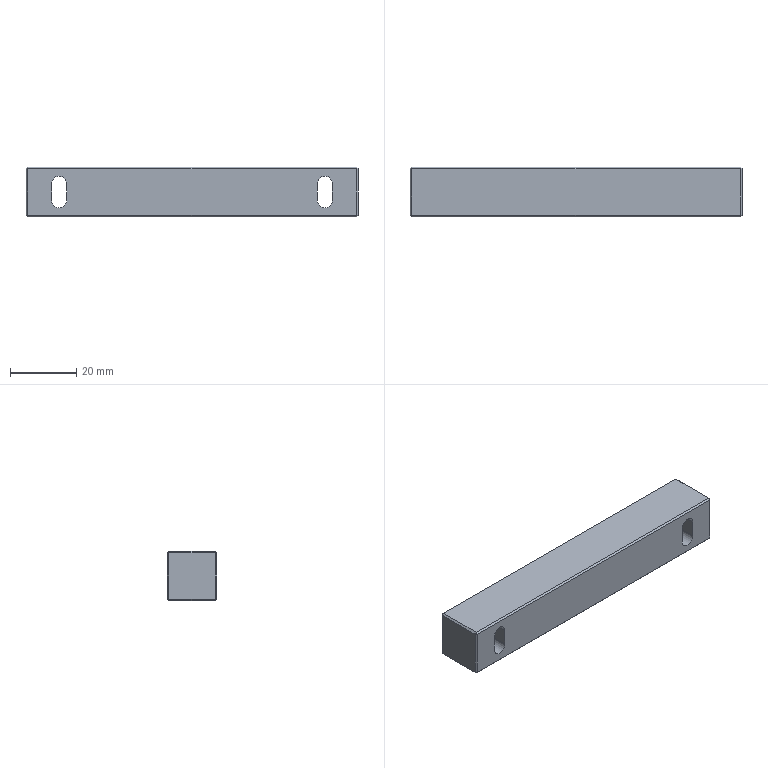Part | SolidWorks | features Chamfer 1, Cut 1, Extrusion 1 | 1 solid | 36 faces | box 100 x 15 x 15 mm | volume 21284 mm3 | plane 30 | cylinder 6 | commonest cylinder face diameters 4.5 x6
STEP:
#1=CARTESIAN_POINT('',(40.,0.,4.75));
#2=VERTEX_POINT('',#1);
#3=CARTESIAN_POINT('',(42.25,0.,2.5));
#4=VERTEX_POINT('',#3);
#5=CARTESIAN_POINT('',(40.,0.,2.5));
#6=DIRECTION('',(0.,1.,0.));
#7=DIRECTION('',(0.,0.,1.));
#8=AXIS2_PLACEMENT_3D('',#5,#6,#7);
#9=CIRCLE('',#8,2.25);
#10=EDGE_CURVE('',#2,#4,#9,.T.);
#11=ORIENTED_EDGE('',*,*,#10,.F.);
#12=CARTESIAN_POINT('',(40.,15.,4.75));
#13=VERTEX_POINT('',#12);
#14=CARTESIAN_POINT('',(40.,0.,4.75));
#15=DIRECTION('',(0.,1.,0.));
#16=VECTOR('',#15,1000.);
#17=LINE('',#14,#16);
#18=EDGE_CURVE('',#2,#13,#17,.T.);
#19=ORIENTED_EDGE('',*,*,#18,.T.);
#20=CARTESIAN_POINT('',(42.25,15.,2.5));
#21=VERTEX_POINT('',#20);
#22=CARTESIAN_POINT('',(40.,15.,2.5));
#23=DIRECTION('',(0.,1.,0.));
#24=DIRECTION('',(0.,0.,1.));
#25=AXIS2_PLACEMENT_3D('',#22,#23,#24);
#26=CIRCLE('',#25,2.25);
#27=EDGE_CURVE('',#13,#21,#26,.T.);
#28=ORIENTED_EDGE('',*,*,#27,.T.);
#29=CARTESIAN_POINT('',(42.25,0.,2.5));
#30=DIRECTION('',(0.,1.,0.));
#31=VECTOR('',#30,1000.);
#32=LINE('',#29,#31);
#33=EDGE_CURVE('',#4,#21,#32,.T.);
#34=ORIENTED_EDGE('',*,*,#33,.F.);
#35=EDGE_LOOP('',(#11,#19,#28,#34));
#36=FACE_OUTER_BOUND('',#35,.T.);
#37=CARTESIAN_POINT('',(40.,0.,2.5));
#38=DIRECTION('',(0.,1.,0.));
#39=DIRECTION('',(0.,0.,1.));
#40=AXIS2_PLACEMENT_3D('',#37,#38,#39);
#41=CYLINDRICAL_SURFACE('',#40,2.25);
#42=ADVANCED_FACE('',(#36),#41,.F.);
#43=CARTESIAN_POINT('',(-40.,0.,4.75));
#44=VERTEX_POINT('',#43);
#45=CARTESIAN_POINT('',(-37.75,0.,2.5));
#46=VERTEX_POINT('',#45);
#47=CARTESIAN_POINT('',(-40.,0.,2.5));
#48=DIRECTION('',(0.,1.,0.));
#49=DIRECTION('',(0.,0.,-1.));
#50=AXIS2_PLACEMENT_3D('',#47,#48,#49);
#51=CIRCLE('',#50,2.25);
#52=EDGE_CURVE('',#44,#46,#51,.T.);
#53=ORIENTED_EDGE('',*,*,#52,.F.);
#54=CARTESIAN_POINT('',(-40.,15.,4.75));
#55=VERTEX_POINT('',#54);
#56=CARTESIAN_POINT('',(-40.,0.,4.75));
#57=DIRECTION('',(0.,1.,0.));
#58=VECTOR('',#57,1000.);
#59=LINE('',#56,#58);
#60=EDGE_CURVE('',#44,#55,#59,.T.);
#61=ORIENTED_EDGE('',*,*,#60,.T.);
#62=CARTESIAN_POINT('',(-37.75,15.,2.5));
#63=VERTEX_POINT('',#62);
#64=CARTESIAN_POINT('',(-40.,15.,2.5));
#65=DIRECTION('',(0.,1.,0.));
#66=DIRECTION('',(0.,0.,-1.));
#67=AXIS2_PLACEMENT_3D('',#64,#65,#66);
#68=CIRCLE('',#67,2.25);
#69=EDGE_CURVE('',#55,#63,#68,.T.);
#70=ORIENTED_EDGE('',*,*,#69,.T.);
#71=CARTESIAN_POINT('',(-37.75,0.,2.5));
#72=DIRECTION('',(0.,1.,0.));
#73=VECTOR('',#72,1000.);
#74=LINE('',#71,#73);
#75=EDGE_CURVE('',#46,#63,#74,.T.);
#76=ORIENTED_EDGE('',*,*,#75,.F.);
#77=EDGE_LOOP('',(#53,#61,#70,#76));
#78=FACE_OUTER_BOUND('',#77,.T.);
#79=CARTESIAN_POINT('',(-40.,0.,2.5));
#80=DIRECTION('',(0.,1.,0.));
#81=DIRECTION('',(0.,0.,1.));
#82=AXIS2_PLACEMENT_3D('',#79,#80,#81);
#83=CYLINDRICAL_SURFACE('',#82,2.25);
#84=ADVANCED_FACE('',(#78),#83,.F.);
#85=CARTESIAN_POINT('',(-50.,14.5,7.));
#86=VERTEX_POINT('',#85);
#87=CARTESIAN_POINT('',(-50.,14.5,-7.));
#88=VERTEX_POINT('',#87);
#89=CARTESIAN_POINT('',(-50.,14.5,-7.5));
#90=DIRECTION('',(0.,0.,-1.));
#91=VECTOR('',#90,1000.);
#92=LINE('',#89,#91);
#93=EDGE_CURVE('',#86,#88,#92,.T.);
#94=ORIENTED_EDGE('',*,*,#93,.T.);
#95=CARTESIAN_POINT('',(-50.,0.5,-7.));
#96=VERTEX_POINT('',#95);
#97=CARTESIAN_POINT('',(-50.,15.,-7.));
#98=DIRECTION('',(0.,-1.,0.));
#99=VECTOR('',#98,1000.);
#100=LINE('',#97,#99);
#101=EDGE_CURVE('',#88,#96,#100,.T.);
#102=ORIENTED_EDGE('',*,*,#101,.T.);
#103=CARTESIAN_POINT('',(-50.,0.5,7.));
#104=VERTEX_POINT('',#103);
#105=CARTESIAN_POINT('',(-50.,0.5,-7.5));
#106=DIRECTION('',(0.,0.,1.));
#107=VECTOR('',#106,1000.);
#108=LINE('',#105,#107);
#109=EDGE_CURVE('',#96,#104,#108,.T.);
#110=ORIENTED_EDGE('',*,*,#109,.T.);
#111=CARTESIAN_POINT('',(-50.,15.,7.));
#112=DIRECTION('',(0.,1.,0.));
#113=VECTOR('',#112,1000.);
#114=LINE('',#111,#113);
#115=EDGE_CURVE('',#104,#86,#114,.T.);
#116=ORIENTED_EDGE('',*,*,#115,.T.);
#117=EDGE_LOOP('',(#94,#102,#110,#116));
#118=FACE_OUTER_BOUND('',#117,.T.);
#119=CARTESIAN_POINT('',(-50.,15.,-7.5));
#120=DIRECTION('',(1.,0.,0.));
#121=DIRECTION('',(0.,0.,-1.));
#122=AXIS2_PLACEMENT_3D('',#119,#120,#121);
#123=PLANE('',#122);
#124=ADVANCED_FACE('',(#118),#123,.F.);
#125=CARTESIAN_POINT('',(49.5,14.5,7.5));
#126=VERTEX_POINT('',#125);
#127=CARTESIAN_POINT('',(-49.5,14.5,7.5));
#128=VERTEX_POINT('',#127);
#129=CARTESIAN_POINT('',(-50.,14.5,7.5));
#130=DIRECTION('',(-1.,0.,0.));
#131=VECTOR('',#130,1000.);
#132=LINE('',#129,#131);
#133=EDGE_CURVE('',#126,#128,#132,.T.);
#134=ORIENTED_EDGE('',*,*,#133,.T.);
#135=CARTESIAN_POINT('',(-49.5,0.5,7.5));
#136=VERTEX_POINT('',#135);
#137=CARTESIAN_POINT('',(-49.5,15.,7.5));
#138=DIRECTION('',(0.,-1.,0.));
#139=VECTOR('',#138,1000.);
#140=LINE('',#137,#139);
#141=EDGE_CURVE('',#128,#136,#140,.T.);
#142=ORIENTED_EDGE('',*,*,#141,.T.);
#143=CARTESIAN_POINT('',(49.5,0.5,7.5));
#144=VERTEX_POINT('',#143);
#145=CARTESIAN_POINT('',(-50.,0.5,7.5));
#146=DIRECTION('',(1.,0.,0.));
#147=VECTOR('',#146,1000.);
#148=LINE('',#145,#147);
#149=EDGE_CURVE('',#136,#144,#148,.T.);
#150=ORIENTED_EDGE('',*,*,#149,.T.);
#151=CARTESIAN_POINT('',(49.5,15.,7.5));
#152=DIRECTION('',(0.,1.,0.));
#153=VECTOR('',#152,1000.);
#154=LINE('',#151,#153);
#155=EDGE_CURVE('',#144,#126,#154,.T.);
#156=ORIENTED_EDGE('',*,*,#155,.T.);
#157=EDGE_LOOP('',(#134,#142,#150,#156));
#158=FACE_OUTER_BOUND('',#157,.T.);
#159=CARTESIAN_POINT('',(-50.,15.,7.5));
#160=DIRECTION('',(0.,0.,-1.));
#161=DIRECTION('',(-1.,0.,0.));
#162=AXIS2_PLACEMENT_3D('',#159,#160,#161);
#163=PLANE('',#162);
#164=ADVANCED_FACE('',(#158),#163,.F.);
#165=CARTESIAN_POINT('',(50.,0.5,-7.));
#166=VERTEX_POINT('',#165);
#167=CARTESIAN_POINT('',(50.,14.5,-7.));
#168=VERTEX_POINT('',#167);
#169=CARTESIAN_POINT('',(50.,15.,-7.));
#170=DIRECTION('',(0.,1.,0.));
#171=VECTOR('',#170,1000.);
#172=LINE('',#169,#171);
#173=EDGE_CURVE('',#166,#168,#172,.T.);
#174=ORIENTED_EDGE('',*,*,#173,.T.);
#175=CARTESIAN_POINT('',(50.,14.5,7.));
#176=VERTEX_POINT('',#175);
#177=CARTESIAN_POINT('',(50.,14.5,7.5));
#178=DIRECTION('',(0.,0.,1.));
#179=VECTOR('',#178,1000.);
#180=LINE('',#177,#179);
#181=EDGE_CURVE('',#168,#176,#180,.T.);
#182=ORIENTED_EDGE('',*,*,#181,.T.);
#183=CARTESIAN_POINT('',(50.,0.5,7.));
#184=VERTEX_POINT('',#183);
#185=CARTESIAN_POINT('',(50.,15.,7.));
#186=DIRECTION('',(0.,-1.,0.));
#187=VECTOR('',#186,1000.);
#188=LINE('',#185,#187);
#189=EDGE_CURVE('',#176,#184,#188,.T.);
#190=ORIENTED_EDGE('',*,*,#189,.T.);
#191=CARTESIAN_POINT('',(50.,0.5,-7.5));
#192=DIRECTION('',(0.,0.,-1.));
#193=VECTOR('',#192,1000.);
#194=LINE('',#191,#193);
#195=EDGE_CURVE('',#184,#166,#194,.T.);
#196=ORIENTED_EDGE('',*,*,#195,.T.);
#197=EDGE_LOOP('',(#174,#182,#190,#196));
#198=FACE_OUTER_BOUND('',#197,.T.);
#199=CARTESIAN_POINT('',(50.,15.,-7.5));
#200=DIRECTION('',(-1.,0.,0.));
#201=DIRECTION('',(0.,0.,1.));
#202=AXIS2_PLACEMENT_3D('',#199,#200,#201);
#203=PLANE('',#202);
#204=ADVANCED_FACE('',(#198),#203,.F.);
#205=CARTESIAN_POINT('',(-49.5,0.5,-7.5));
#206=VERTEX_POINT('',#205);
#207=CARTESIAN_POINT('',(-49.5,14.5,-7.5));
#208=VERTEX_POINT('',#207);
#209=CARTESIAN_POINT('',(-49.5,15.,-7.5));
#210=DIRECTION('',(0.,1.,0.));
#211=VECTOR('',#210,1000.);
#212=LINE('',#209,#211);
#213=EDGE_CURVE('',#206,#208,#212,.T.);
#214=ORIENTED_EDGE('',*,*,#213,.T.);
#215=CARTESIAN_POINT('',(49.5,14.5,-7.5));
#216=VERTEX_POINT('',#215);
#217=CARTESIAN_POINT('',(50.,14.5,-7.5));
#218=DIRECTION('',(1.,0.,0.));
#219=VECTOR('',#218,1000.);
#220=LINE('',#217,#219);
#221=EDGE_CURVE('',#208,#216,#220,.T.);
#222=ORIENTED_EDGE('',*,*,#221,.T.);
#223=CARTESIAN_POINT('',(49.5,0.5,-7.5));
#224=VERTEX_POINT('',#223);
#225=CARTESIAN_POINT('',(49.5,15.,-7.5));
#226=DIRECTION('',(0.,-1.,0.));
#227=VECTOR('',#226,1000.);
#228=LINE('',#225,#227);
#229=EDGE_CURVE('',#216,#224,#228,.T.);
#230=ORIENTED_EDGE('',*,*,#229,.T.);
#231=CARTESIAN_POINT('',(-50.,0.5,-7.5));
#232=DIRECTION('',(-1.,0.,0.));
#233=VECTOR('',#232,1000.);
#234=LINE('',#231,#233);
#235=EDGE_CURVE('',#224,#206,#234,.T.);
#236=ORIENTED_EDGE('',*,*,#235,.T.);
#237=EDGE_LOOP('',(#214,#222,#230,#236));
#238=FACE_OUTER_BOUND('',#237,.T.);
#239=CARTESIAN_POINT('',(-50.,15.,-7.5));
#240=DIRECTION('',(0.,0.,1.));
#241=DIRECTION('',(1.,0.,0.));
#242=AXIS2_PLACEMENT_3D('',#239,#240,#241);
#243=PLANE('',#242);
#244=ADVANCED_FACE('',(#238),#243,.F.);
#245=CARTESIAN_POINT('',(49.5,15.,-7.));
#246=VERTEX_POINT('',#245);
#247=CARTESIAN_POINT('',(-49.5,15.,-7.));
#248=VERTEX_POINT('',#247);
#249=CARTESIAN_POINT('',(-50.,15.,-7.));
#250=DIRECTION('',(-1.,0.,0.));
#251=VECTOR('',#250,1000.);
#252=LINE('',#249,#251);
#253=EDGE_CURVE('',#246,#248,#252,.T.);
#254=ORIENTED_EDGE('',*,*,#253,.T.);
#255=CARTESIAN_POINT('',(-49.5,15.,7.));
#256=VERTEX_POINT('',#255);
#257=CARTESIAN_POINT('',(-49.5,15.,7.5));
#258=DIRECTION('',(0.,0.,1.));
#259=VECTOR('',#258,1000.);
#260=LINE('',#257,#259);
#261=EDGE_CURVE('',#248,#256,#260,.T.);
#262=ORIENTED_EDGE('',*,*,#261,.T.);
#263=CARTESIAN_POINT('',(49.5,15.,7.));
#264=VERTEX_POINT('',#263);
#265=CARTESIAN_POINT('',(50.,15.,7.));
#266=DIRECTION('',(1.,0.,0.));
#267=VECTOR('',#266,1000.);
#268=LINE('',#265,#267);
#269=EDGE_CURVE('',#256,#264,#268,.T.);
#270=ORIENTED_EDGE('',*,*,#269,.T.);
#271=CARTESIAN_POINT('',(49.5,15.,-7.5));
#272=DIRECTION('',(0.,0.,-1.));
#273=VECTOR('',#272,1000.);
#274=LINE('',#271,#273);
#275=EDGE_CURVE('',#264,#246,#274,.T.);
#276=ORIENTED_EDGE('',*,*,#275,.T.);
#277=EDGE_LOOP('',(#254,#262,#270,#276));
#278=FACE_OUTER_BOUND('',#277,.T.);
#279=CARTESIAN_POINT('',(37.75,15.,2.5));
#280=VERTEX_POINT('',#279);
#281=CARTESIAN_POINT('',(40.,15.,2.5));
#282=DIRECTION('',(0.,1.,0.));
#283=DIRECTION('',(0.,0.,1.));
#284=AXIS2_PLACEMENT_3D('',#281,#282,#283);
#285=CIRCLE('',#284,2.25);
#286=EDGE_CURVE('',#280,#13,#285,.T.);
#287=ORIENTED_EDGE('',*,*,#286,.F.);
#288=CARTESIAN_POINT('',(37.75,15.,-2.5));
#289=VERTEX_POINT('',#288);
#290=CARTESIAN_POINT('',(37.75,15.,-2.5));
#291=DIRECTION('',(0.,0.,1.));
#292=VECTOR('',#291,1000.);
#293=LINE('',#290,#292);
#294=EDGE_CURVE('',#289,#280,#293,.T.);
#295=ORIENTED_EDGE('',*,*,#294,.F.);
#296=CARTESIAN_POINT('',(42.25,15.,-2.5));
#297=VERTEX_POINT('',#296);
#298=CARTESIAN_POINT('',(40.,15.,-2.5));
#299=DIRECTION('',(0.,1.,0.));
#300=DIRECTION('',(0.,0.,1.));
#301=AXIS2_PLACEMENT_3D('',#298,#299,#300);
#302=CIRCLE('',#301,2.25);
#303=EDGE_CURVE('',#297,#289,#302,.T.);
#304=ORIENTED_EDGE('',*,*,#303,.F.);
#305=CARTESIAN_POINT('',(42.25,15.,-2.5));
#306=DIRECTION('',(0.,0.,-1.));
#307=VECTOR('',#306,1000.);
#308=LINE('',#305,#307);
#309=EDGE_CURVE('',#21,#297,#308,.T.);
#310=ORIENTED_EDGE('',*,*,#309,.F.);
#311=ORIENTED_EDGE('',*,*,#27,.F.);
#312=EDGE_LOOP('',(#287,#295,#304,#310,#311));
#313=FACE_BOUND('',#312,.T.);
#314=CARTESIAN_POINT('',(-37.75,15.,-2.5));
#315=VERTEX_POINT('',#314);
#316=CARTESIAN_POINT('',(-42.25,15.,-2.5));
#317=VERTEX_POINT('',#316);
#318=CARTESIAN_POINT('',(-40.,15.,-2.5));
#319=DIRECTION('',(0.,1.,0.));
#320=DIRECTION('',(0.,0.,-1.));
#321=AXIS2_PLACEMENT_3D('',#318,#319,#320);
#322=CIRCLE('',#321,2.25);
#323=EDGE_CURVE('',#315,#317,#322,.T.);
#324=ORIENTED_EDGE('',*,*,#323,.F.);
#325=CARTESIAN_POINT('',(-37.75,15.,-2.5));
#326=DIRECTION('',(0.,0.,-1.));
#327=VECTOR('',#326,1000.);
#328=LINE('',#325,#327);
#329=EDGE_CURVE('',#63,#315,#328,.T.);
#330=ORIENTED_EDGE('',*,*,#329,.F.);
#331=ORIENTED_EDGE('',*,*,#69,.F.);
#332=CARTESIAN_POINT('',(-42.25,15.,2.5));
#333=VERTEX_POINT('',#332);
#334=CARTESIAN_POINT('',(-40.,15.,2.5));
#335=DIRECTION('',(0.,1.,0.));
#336=DIRECTION('',(0.,0.,-1.));
#337=AXIS2_PLACEMENT_3D('',#334,#335,#336);
#338=CIRCLE('',#337,2.25);
#339=EDGE_CURVE('',#333,#55,#338,.T.);
#340=ORIENTED_EDGE('',*,*,#339,.F.);
#341=CARTESIAN_POINT('',(-42.25,15.,-2.5));
#342=DIRECTION('',(0.,0.,1.));
#343=VECTOR('',#342,1000.);
#344=LINE('',#341,#343);
#345=EDGE_CURVE('',#317,#333,#344,.T.);
#346=ORIENTED_EDGE('',*,*,#345,.F.);
#347=EDGE_LOOP('',(#324,#330,#331,#340,#346));
#348=FACE_BOUND('',#347,.T.);
#349=CARTESIAN_POINT('',(-50.,15.,-7.5));
#350=DIRECTION('',(0.,1.,0.));
#351=DIRECTION('',(0.,0.,1.));
#352=AXIS2_PLACEMENT_3D('',#349,#350,#351);
#353=PLANE('',#352);
#354=ADVANCED_FACE('',(#278,#313,#348),#353,.T.);
#355=CARTESIAN_POINT('',(49.5,0.,7.));
#356=VERTEX_POINT('',#355);
#357=CARTESIAN_POINT('',(-49.5,0.,7.));
#358=VERTEX_POINT('',#357);
#359=CARTESIAN_POINT('',(-50.,0.,7.));
#360=DIRECTION('',(-1.,0.,0.));
#361=VECTOR('',#360,1000.);
#362=LINE('',#359,#361);
#363=EDGE_CURVE('',#356,#358,#362,.T.);
#364=ORIENTED_EDGE('',*,*,#363,.T.);
#365=CARTESIAN_POINT('',(-49.5,0.,-7.));
#366=VERTEX_POINT('',#365);
#367=CARTESIAN_POINT('',(-49.5,0.,-7.5));
#368=DIRECTION('',(0.,0.,-1.));
#369=VECTOR('',#368,1000.);
#370=LINE('',#367,#369);
#371=EDGE_CURVE('',#358,#366,#370,.T.);
#372=ORIENTED_EDGE('',*,*,#371,.T.);
#373=CARTESIAN_POINT('',(49.5,0.,-7.));
#374=VERTEX_POINT('',#373);
#375=CARTESIAN_POINT('',(-50.,0.,-7.));
#376=DIRECTION('',(1.,0.,0.));
#377=VECTOR('',#376,1000.);
#378=LINE('',#375,#377);
#379=EDGE_CURVE('',#366,#374,#378,.T.);
#380=ORIENTED_EDGE('',*,*,#379,.T.);
#381=CARTESIAN_POINT('',(49.5,0.,-7.5));
#382=DIRECTION('',(0.,0.,1.));
#383=VECTOR('',#382,1000.);
#384=LINE('',#381,#383);
#385=EDGE_CURVE('',#374,#356,#384,.T.);
#386=ORIENTED_EDGE('',*,*,#385,.T.);
#387=EDGE_LOOP('',(#364,#372,#380,#386));
#388=FACE_OUTER_BOUND('',#387,.T.);
#389=CARTESIAN_POINT('',(37.75,0.,-2.5));
#390=VERTEX_POINT('',#389);
#391=CARTESIAN_POINT('',(37.75,0.,2.5));
#392=VERTEX_POINT('',#391);
#393=CARTESIAN_POINT('',(37.75,0.,-2.5));
#394=DIRECTION('',(0.,0.,1.));
#395=VECTOR('',#394,1000.);
#396=LINE('',#393,#395);
#397=EDGE_CURVE('',#390,#392,#396,.T.);
#398=ORIENTED_EDGE('',*,*,#397,.T.);
#399=CARTESIAN_POINT('',(40.,0.,2.5));
#400=DIRECTION('',(0.,1.,0.));
#401=DIRECTION('',(0.,0.,1.));
#402=AXIS2_PLACEMENT_3D('',#399,#400,#401);
#403=CIRCLE('',#402,2.25);
#404=EDGE_CURVE('',#392,#2,#403,.T.);
#405=ORIENTED_EDGE('',*,*,#404,.T.);
#406=ORIENTED_EDGE('',*,*,#10,.T.);
#407=CARTESIAN_POINT('',(42.25,0.,-2.5));
#408=VERTEX_POINT('',#407);
#409=CARTESIAN_POINT('',(42.25,0.,-2.5));
#410=DIRECTION('',(0.,0.,-1.));
#411=VECTOR('',#410,1000.);
#412=LINE('',#409,#411);
#413=EDGE_CURVE('',#4,#408,#412,.T.);
#414=ORIENTED_EDGE('',*,*,#413,.T.);
#415=CARTESIAN_POINT('',(40.,0.,-2.5));
#416=DIRECTION('',(0.,1.,0.));
#417=DIRECTION('',(0.,0.,1.));
#418=AXIS2_PLACEMENT_3D('',#415,#416,#417);
#419=CIRCLE('',#418,2.25);
#420=EDGE_CURVE('',#408,#390,#419,.T.);
#421=ORIENTED_EDGE('',*,*,#420,.T.);
#422=EDGE_LOOP('',(#398,#405,#406,#414,#421));
#423=FACE_BOUND('',#422,.T.);
#424=CARTESIAN_POINT('',(-37.75,0.,-2.5));
#425=VERTEX_POINT('',#424);
#426=CARTESIAN_POINT('',(-37.75,0.,-2.5));
#427=DIRECTION('',(0.,0.,-1.));
#428=VECTOR('',#427,1000.);
#429=LINE('',#426,#428);
#430=EDGE_CURVE('',#46,#425,#429,.T.);
#431=ORIENTED_EDGE('',*,*,#430,.T.);
#432=CARTESIAN_POINT('',(-42.25,0.,-2.5));
#433=VERTEX_POINT('',#432);
#434=CARTESIAN_POINT('',(-40.,0.,-2.5));
#435=DIRECTION('',(0.,1.,0.));
#436=DIRECTION('',(0.,0.,-1.));
#437=AXIS2_PLACEMENT_3D('',#434,#435,#436);
#438=CIRCLE('',#437,2.25);
#439=EDGE_CURVE('',#425,#433,#438,.T.);
#440=ORIENTED_EDGE('',*,*,#439,.T.);
#441=CARTESIAN_POINT('',(-42.25,0.,2.5));
#442=VERTEX_POINT('',#441);
#443=CARTESIAN_POINT('',(-42.25,0.,-2.5));
#444=DIRECTION('',(0.,0.,1.));
#445=VECTOR('',#444,1000.);
#446=LINE('',#443,#445);
#447=EDGE_CURVE('',#433,#442,#446,.T.);
#448=ORIENTED_EDGE('',*,*,#447,.T.);
#449=CARTESIAN_POINT('',(-40.,0.,2.5));
#450=DIRECTION('',(0.,1.,0.));
#451=DIRECTION('',(0.,0.,-1.));
#452=AXIS2_PLACEMENT_3D('',#449,#450,#451);
#453=CIRCLE('',#452,2.25);
#454=EDGE_CURVE('',#442,#44,#453,.T.);
#455=ORIENTED_EDGE('',*,*,#454,.T.);
#456=ORIENTED_EDGE('',*,*,#52,.T.);
#457=EDGE_LOOP('',(#431,#440,#448,#455,#456));
#458=FACE_BOUND('',#457,.T.);
#459=CARTESIAN_POINT('',(-50.,0.,-7.5));
#460=DIRECTION('',(0.,1.,0.));
#461=DIRECTION('',(0.,0.,1.));
#462=AXIS2_PLACEMENT_3D('',#459,#460,#461);
#463=PLANE('',#462);
#464=ADVANCED_FACE('',(#388,#423,#458),#463,.F.);
#465=ORIENTED_EDGE('',*,*,#323,.T.);
#466=CARTESIAN_POINT('',(-42.25,0.,-2.5));
#467=DIRECTION('',(0.,1.,0.));
#468=VECTOR('',#467,1000.);
#469=LINE('',#466,#468);
#470=EDGE_CURVE('',#433,#317,#469,.T.);
#471=ORIENTED_EDGE('',*,*,#470,.F.);
#472=ORIENTED_EDGE('',*,*,#439,.F.);
#473=CARTESIAN_POINT('',(-37.75,0.,-2.5));
#474=DIRECTION('',(0.,1.,0.));
#475=VECTOR('',#474,1000.);
#476=LINE('',#473,#475);
#477=EDGE_CURVE('',#425,#315,#476,.T.);
#478=ORIENTED_EDGE('',*,*,#477,.T.);
#479=EDGE_LOOP('',(#465,#471,#472,#478));
#480=FACE_OUTER_BOUND('',#479,.T.);
#481=CARTESIAN_POINT('',(-40.,0.,-2.5));
#482=DIRECTION('',(0.,1.,0.));
#483=DIRECTION('',(0.,0.,1.));
#484=AXIS2_PLACEMENT_3D('',#481,#482,#483);
#485=CYLINDRICAL_SURFACE('',#484,2.25);
#486=ADVANCED_FACE('',(#480),#485,.F.);
#487=ORIENTED_EDGE('',*,*,#329,.T.);
#488=ORIENTED_EDGE('',*,*,#477,.F.);
#489=ORIENTED_EDGE('',*,*,#430,.F.);
#490=ORIENTED_EDGE('',*,*,#75,.T.);
#491=EDGE_LOOP('',(#487,#488,#489,#490));
#492=FACE_OUTER_BOUND('',#491,.T.);
#493=CARTESIAN_POINT('',(-37.75,0.,-2.5));
#494=DIRECTION('',(1.,0.,0.));
#495=DIRECTION('',(0.,0.,-1.));
#496=AXIS2_PLACEMENT_3D('',#493,#494,#495);
#497=PLANE('',#496);
#498=ADVANCED_FACE('',(#492),#497,.F.);
#499=ORIENTED_EDGE('',*,*,#60,.F.);
#500=ORIENTED_EDGE('',*,*,#454,.F.);
#501=CARTESIAN_POINT('',(-42.25,0.,2.5));
#502=DIRECTION('',(0.,1.,0.));
#503=VECTOR('',#502,1000.);
#504=LINE('',#501,#503);
#505=EDGE_CURVE('',#442,#333,#504,.T.);
#506=ORIENTED_EDGE('',*,*,#505,.T.);
#507=ORIENTED_EDGE('',*,*,#339,.T.);
#508=EDGE_LOOP('',(#499,#500,#506,#507));
#509=FACE_OUTER_BOUND('',#508,.T.);
#510=CARTESIAN_POINT('',(-40.,0.,2.5));
#511=DIRECTION('',(0.,1.,0.));
#512=DIRECTION('',(0.,0.,1.));
#513=AXIS2_PLACEMENT_3D('',#510,#511,#512);
#514=CYLINDRICAL_SURFACE('',#513,2.25);
#515=ADVANCED_FACE('',(#509),#514,.F.);
#516=ORIENTED_EDGE('',*,*,#345,.T.);
#517=ORIENTED_EDGE('',*,*,#505,.F.);
#518=ORIENTED_EDGE('',*,*,#447,.F.);
#519=ORIENTED_EDGE('',*,*,#470,.T.);
#520=EDGE_LOOP('',(#516,#517,#518,#519));
#521=FACE_OUTER_BOUND('',#520,.T.);
#522=CARTESIAN_POINT('',(-42.25,0.,-2.5));
#523=DIRECTION('',(-1.,0.,0.));
#524=DIRECTION('',(0.,0.,1.));
#525=AXIS2_PLACEMENT_3D('',#522,#523,#524);
#526=PLANE('',#525);
#527=ADVANCED_FACE('',(#521),#526,.F.);
#528=ORIENTED_EDGE('',*,*,#18,.F.);
#529=ORIENTED_EDGE('',*,*,#404,.F.);
#530=CARTESIAN_POINT('',(37.75,0.,2.5));
#531=DIRECTION('',(0.,1.,0.));
#532=VECTOR('',#531,1000.);
#533=LINE('',#530,#532);
#534=EDGE_CURVE('',#392,#280,#533,.T.);
#535=ORIENTED_EDGE('',*,*,#534,.T.);
#536=ORIENTED_EDGE('',*,*,#286,.T.);
#537=EDGE_LOOP('',(#528,#529,#535,#536));
#538=FACE_OUTER_BOUND('',#537,.T.);
#539=CARTESIAN_POINT('',(40.,0.,2.5));
#540=DIRECTION('',(0.,1.,0.));
#541=DIRECTION('',(0.,0.,1.));
#542=AXIS2_PLACEMENT_3D('',#539,#540,#541);
#543=CYLINDRICAL_SURFACE('',#542,2.25);
#544=ADVANCED_FACE('',(#538),#543,.F.);
#545=ORIENTED_EDGE('',*,*,#294,.T.);
#546=ORIENTED_EDGE('',*,*,#534,.F.);
#547=ORIENTED_EDGE('',*,*,#397,.F.);
#548=CARTESIAN_POINT('',(37.75,0.,-2.5));
#549=DIRECTION('',(0.,1.,0.));
#550=VECTOR('',#549,1000.);
#551=LINE('',#548,#550);
#552=EDGE_CURVE('',#390,#289,#551,.T.);
#553=ORIENTED_EDGE('',*,*,#552,.T.);
#554=EDGE_LOOP('',(#545,#546,#547,#553));
#555=FACE_OUTER_BOUND('',#554,.T.);
#556=CARTESIAN_POINT('',(37.75,0.,-2.5));
#557=DIRECTION('',(-1.,0.,0.));
#558=DIRECTION('',(0.,0.,1.));
#559=AXIS2_PLACEMENT_3D('',#556,#557,#558);
#560=PLANE('',#559);
#561=ADVANCED_FACE('',(#555),#560,.F.);
#562=ORIENTED_EDGE('',*,*,#303,.T.);
#563=ORIENTED_EDGE('',*,*,#552,.F.);
#564=ORIENTED_EDGE('',*,*,#420,.F.);
#565=CARTESIAN_POINT('',(42.25,0.,-2.5));
#566=DIRECTION('',(0.,1.,0.));
#567=VECTOR('',#566,1000.);
#568=LINE('',#565,#567);
#569=EDGE_CURVE('',#408,#297,#568,.T.);
#570=ORIENTED_EDGE('',*,*,#569,.T.);
#571=EDGE_LOOP('',(#562,#563,#564,#570));
#572=FACE_OUTER_BOUND('',#571,.T.);
#573=CARTESIAN_POINT('',(40.,0.,-2.5));
#574=DIRECTION('',(0.,1.,0.));
#575=DIRECTION('',(0.,0.,1.));
#576=AXIS2_PLACEMENT_3D('',#573,#574,#575);
#577=CYLINDRICAL_SURFACE('',#576,2.25);
#578=ADVANCED_FACE('',(#572),#577,.F.);
#579=ORIENTED_EDGE('',*,*,#309,.T.);
#580=ORIENTED_EDGE('',*,*,#569,.F.);
#581=ORIENTED_EDGE('',*,*,#413,.F.);
#582=ORIENTED_EDGE('',*,*,#33,.T.);
#583=EDGE_LOOP('',(#579,#580,#581,#582));
#584=FACE_OUTER_BOUND('',#583,.T.);
#585=CARTESIAN_POINT('',(42.25,0.,-2.5));
#586=DIRECTION('',(1.,0.,0.));
#587=DIRECTION('',(0.,0.,-1.));
#588=AXIS2_PLACEMENT_3D('',#585,#586,#587);
#589=PLANE('',#588);
#590=ADVANCED_FACE('',(#584),#589,.F.);
#591=CARTESIAN_POINT('',(49.5,0.,-7.));
#592=DIRECTION('',(-0.7071,-0.7071,0.));
#593=VECTOR('',#592,1000.);
#594=LINE('',#591,#593);
#595=EDGE_CURVE('',#166,#374,#594,.T.);
#596=ORIENTED_EDGE('',*,*,#595,.F.);
#597=ORIENTED_EDGE('',*,*,#195,.F.);
#598=CARTESIAN_POINT('',(49.5,0.,7.));
#599=DIRECTION('',(0.7071,0.7071,0.));
#600=VECTOR('',#599,1000.);
#601=LINE('',#598,#600);
#602=EDGE_CURVE('',#356,#184,#601,.T.);
#603=ORIENTED_EDGE('',*,*,#602,.F.);
#604=ORIENTED_EDGE('',*,*,#385,.F.);
#605=EDGE_LOOP('',(#596,#597,#603,#604));
#606=FACE_OUTER_BOUND('',#605,.T.);
#607=CARTESIAN_POINT('',(50.,0.5,-7.5));
#608=DIRECTION('',(-0.7071,0.7071,0.));
#609=DIRECTION('',(-0.7071,-0.7071,0.));
#610=AXIS2_PLACEMENT_3D('',#607,#608,#609);
#611=PLANE('',#610);
#612=ADVANCED_FACE('',(#606),#611,.F.);
#613=CARTESIAN_POINT('',(49.75,0.5,-7.25));
#614=DIRECTION('',(-0.7071,0.,-0.7071));
#615=VECTOR('',#614,1000.);
#616=LINE('',#613,#615);
#617=EDGE_CURVE('',#166,#224,#616,.T.);
#618=ORIENTED_EDGE('',*,*,#617,.F.);
#619=ORIENTED_EDGE('',*,*,#595,.T.);
#620=CARTESIAN_POINT('',(49.5,0.,-7.));
#621=DIRECTION('',(0.,-0.7071,0.7071));
#622=VECTOR('',#621,1000.);
#623=LINE('',#620,#622);
#624=EDGE_CURVE('',#224,#374,#623,.T.);
#625=ORIENTED_EDGE('',*,*,#624,.F.);
#626=EDGE_LOOP('',(#618,#619,#625));
#627=FACE_OUTER_BOUND('',#626,.T.);
#628=CARTESIAN_POINT('',(49.5,0.,-7.));
#629=DIRECTION('',(0.5774,-0.5774,-0.5774));
#630=DIRECTION('',(-0.7071,0.,-0.7071));
#631=AXIS2_PLACEMENT_3D('',#628,#629,#630);
#632=PLANE('',#631);
#633=ADVANCED_FACE('',(#627),#632,.T.);
#634=CARTESIAN_POINT('',(49.5,0.,7.));
#635=DIRECTION('',(0.,0.7071,0.7071));
#636=VECTOR('',#635,1000.);
#637=LINE('',#634,#636);
#638=EDGE_CURVE('',#356,#144,#637,.T.);
#639=ORIENTED_EDGE('',*,*,#638,.F.);
#640=ORIENTED_EDGE('',*,*,#602,.T.);
#641=CARTESIAN_POINT('',(49.75,0.5,7.25));
#642=DIRECTION('',(0.7071,0.,-0.7071));
#643=VECTOR('',#642,1000.);
#644=LINE('',#641,#643);
#645=EDGE_CURVE('',#144,#184,#644,.T.);
#646=ORIENTED_EDGE('',*,*,#645,.F.);
#647=EDGE_LOOP('',(#639,#640,#646));
#648=FACE_OUTER_BOUND('',#647,.T.);
#649=CARTESIAN_POINT('',(49.5,0.,7.));
#650=DIRECTION('',(0.5774,-0.5774,0.5774));
#651=DIRECTION('',(0.,-0.7071,-0.7071));
#652=AXIS2_PLACEMENT_3D('',#649,#650,#651);
#653=PLANE('',#652);
#654=ADVANCED_FACE('',(#648),#653,.T.);
#655=ORIENTED_EDGE('',*,*,#624,.T.);
#656=ORIENTED_EDGE('',*,*,#379,.F.);
#657=CARTESIAN_POINT('',(-49.5,0.,-7.));
#658=DIRECTION('',(0.,-0.7071,0.7071));
#659=VECTOR('',#658,1000.);
#660=LINE('',#657,#659);
#661=EDGE_CURVE('',#206,#366,#660,.T.);
#662=ORIENTED_EDGE('',*,*,#661,.F.);
#663=ORIENTED_EDGE('',*,*,#235,.F.);
#664=EDGE_LOOP('',(#655,#656,#662,#663));
#665=FACE_OUTER_BOUND('',#664,.T.);
#666=CARTESIAN_POINT('',(-50.,0.5,-7.5));
#667=DIRECTION('',(0.,0.7071,0.7071));
#668=DIRECTION('',(0.,-0.7071,0.7071));
#669=AXIS2_PLACEMENT_3D('',#666,#667,#668);
#670=PLANE('',#669);
#671=ADVANCED_FACE('',(#665),#670,.F.);
#672=ORIENTED_EDGE('',*,*,#617,.T.);
#673=ORIENTED_EDGE('',*,*,#229,.F.);
#674=CARTESIAN_POINT('',(49.5,14.5,-7.5));
#675=DIRECTION('',(-0.7071,0.,-0.7071));
#676=VECTOR('',#675,1000.);
#677=LINE('',#674,#676);
#678=EDGE_CURVE('',#168,#216,#677,.T.);
#679=ORIENTED_EDGE('',*,*,#678,.F.);
#680=ORIENTED_EDGE('',*,*,#173,.F.);
#681=EDGE_LOOP('',(#672,#673,#679,#680));
#682=FACE_OUTER_BOUND('',#681,.T.);
#683=CARTESIAN_POINT('',(49.5,15.,-7.5));
#684=DIRECTION('',(-0.7071,0.,0.7071));
#685=DIRECTION('',(0.7071,0.,0.7071));
#686=AXIS2_PLACEMENT_3D('',#683,#684,#685);
#687=PLANE('',#686);
#688=ADVANCED_FACE('',(#682),#687,.F.);
#689=CARTESIAN_POINT('',(50.,14.5,7.));
#690=DIRECTION('',(-0.7071,0.7071,0.));
#691=VECTOR('',#690,1000.);
#692=LINE('',#689,#691);
#693=EDGE_CURVE('',#176,#264,#692,.T.);
#694=ORIENTED_EDGE('',*,*,#693,.F.);
#695=ORIENTED_EDGE('',*,*,#181,.F.);
#696=CARTESIAN_POINT('',(49.75,14.75,-7.));
#697=DIRECTION('',(0.7071,-0.7071,0.));
#698=VECTOR('',#697,1000.);
#699=LINE('',#696,#698);
#700=EDGE_CURVE('',#246,#168,#699,.T.);
#701=ORIENTED_EDGE('',*,*,#700,.F.);
#702=ORIENTED_EDGE('',*,*,#275,.F.);
#703=EDGE_LOOP('',(#694,#695,#701,#702));
#704=FACE_OUTER_BOUND('',#703,.T.);
#705=CARTESIAN_POINT('',(49.5,15.,-7.5));
#706=DIRECTION('',(0.7071,0.7071,0.));
#707=DIRECTION('',(-0.7071,0.7071,0.));
#708=AXIS2_PLACEMENT_3D('',#705,#706,#707);
#709=PLANE('',#708);
#710=ADVANCED_FACE('',(#704),#709,.T.);
#711=ORIENTED_EDGE('',*,*,#645,.T.);
#712=ORIENTED_EDGE('',*,*,#189,.F.);
#713=CARTESIAN_POINT('',(50.,14.5,7.));
#714=DIRECTION('',(0.7071,0.,-0.7071));
#715=VECTOR('',#714,1000.);
#716=LINE('',#713,#715);
#717=EDGE_CURVE('',#126,#176,#716,.T.);
#718=ORIENTED_EDGE('',*,*,#717,.F.);
#719=ORIENTED_EDGE('',*,*,#155,.F.);
#720=EDGE_LOOP('',(#711,#712,#718,#719));
#721=FACE_OUTER_BOUND('',#720,.T.);
#722=CARTESIAN_POINT('',(50.,15.,7.));
#723=DIRECTION('',(-0.7071,0.,-0.7071));
#724=DIRECTION('',(-0.7071,0.,0.7071));
#725=AXIS2_PLACEMENT_3D('',#722,#723,#724);
#726=PLANE('',#725);
#727=ADVANCED_FACE('',(#721),#726,.F.);
#728=ORIENTED_EDGE('',*,*,#638,.T.);
#729=ORIENTED_EDGE('',*,*,#149,.F.);
#730=CARTESIAN_POINT('',(-49.5,0.25,7.25));
#731=DIRECTION('',(0.,0.7071,0.7071));
#732=VECTOR('',#731,1000.);
#733=LINE('',#730,#732);
#734=EDGE_CURVE('',#358,#136,#733,.T.);
#735=ORIENTED_EDGE('',*,*,#734,.F.);
#736=ORIENTED_EDGE('',*,*,#363,.F.);
#737=EDGE_LOOP('',(#728,#729,#735,#736));
#738=FACE_OUTER_BOUND('',#737,.T.);
#739=CARTESIAN_POINT('',(-50.,0.5,7.5));
#740=DIRECTION('',(0.,0.7071,-0.7071));
#741=DIRECTION('',(0.,0.7071,0.7071));
#742=AXIS2_PLACEMENT_3D('',#739,#740,#741);
#743=PLANE('',#742);
#744=ADVANCED_FACE('',(#738),#743,.F.);
#745=CARTESIAN_POINT('',(-49.5,0.,-7.));
#746=DIRECTION('',(-0.7071,0.7071,0.));
#747=VECTOR('',#746,1000.);
#748=LINE('',#745,#747);
#749=EDGE_CURVE('',#366,#96,#748,.T.);
#750=ORIENTED_EDGE('',*,*,#749,.F.);
#751=ORIENTED_EDGE('',*,*,#371,.F.);
#752=CARTESIAN_POINT('',(-50.,0.5,7.));
#753=DIRECTION('',(0.7071,-0.7071,0.));
#754=VECTOR('',#753,1000.);
#755=LINE('',#752,#754);
#756=EDGE_CURVE('',#104,#358,#755,.T.);
#757=ORIENTED_EDGE('',*,*,#756,.F.);
#758=ORIENTED_EDGE('',*,*,#109,.F.);
#759=EDGE_LOOP('',(#750,#751,#757,#758));
#760=FACE_OUTER_BOUND('',#759,.T.);
#761=CARTESIAN_POINT('',(-50.,0.5,-7.5));
#762=DIRECTION('',(0.7071,0.7071,0.));
#763=DIRECTION('',(-0.7071,0.7071,0.));
#764=AXIS2_PLACEMENT_3D('',#761,#762,#763);
#765=PLANE('',#764);
#766=ADVANCED_FACE('',(#760),#765,.F.);
#767=ORIENTED_EDGE('',*,*,#661,.T.);
#768=ORIENTED_EDGE('',*,*,#749,.T.);
#769=CARTESIAN_POINT('',(-49.75,0.5,-7.25));
#770=DIRECTION('',(-0.7071,0.,0.7071));
#771=VECTOR('',#770,1000.);
#772=LINE('',#769,#771);
#773=EDGE_CURVE('',#206,#96,#772,.T.);
#774=ORIENTED_EDGE('',*,*,#773,.F.);
#775=EDGE_LOOP('',(#767,#768,#774));
#776=FACE_OUTER_BOUND('',#775,.T.);
#777=CARTESIAN_POINT('',(-49.5,0.,-7.));
#778=DIRECTION('',(-0.5774,-0.5774,-0.5774));
#779=DIRECTION('',(-0.7071,0.,0.7071));
#780=AXIS2_PLACEMENT_3D('',#777,#778,#779);
#781=PLANE('',#780);
#782=ADVANCED_FACE('',(#776),#781,.T.);
#783=ORIENTED_EDGE('',*,*,#700,.T.);
#784=ORIENTED_EDGE('',*,*,#678,.T.);
#785=CARTESIAN_POINT('',(49.5,14.5,-7.5));
#786=DIRECTION('',(0.,-0.7071,-0.7071));
#787=VECTOR('',#786,1000.);
#788=LINE('',#785,#787);
#789=EDGE_CURVE('',#246,#216,#788,.T.);
#790=ORIENTED_EDGE('',*,*,#789,.F.);
#791=EDGE_LOOP('',(#783,#784,#790));
#792=FACE_OUTER_BOUND('',#791,.T.);
#793=CARTESIAN_POINT('',(49.5,14.5,-7.5));
#794=DIRECTION('',(0.5774,0.5774,-0.5774));
#795=DIRECTION('',(-0.7071,0.,-0.7071));
#796=AXIS2_PLACEMENT_3D('',#793,#794,#795);
#797=PLANE('',#796);
#798=ADVANCED_FACE('',(#792),#797,.T.);
#799=ORIENTED_EDGE('',*,*,#717,.T.);
#800=ORIENTED_EDGE('',*,*,#693,.T.);
#801=CARTESIAN_POINT('',(49.5,14.75,7.25));
#802=DIRECTION('',(0.,0.7071,-0.7071));
#803=VECTOR('',#802,1000.);
#804=LINE('',#801,#803);
#805=EDGE_CURVE('',#126,#264,#804,.T.);
#806=ORIENTED_EDGE('',*,*,#805,.F.);
#807=EDGE_LOOP('',(#799,#800,#806));
#808=FACE_OUTER_BOUND('',#807,.T.);
#809=CARTESIAN_POINT('',(50.,14.5,7.));
#810=DIRECTION('',(0.5774,0.5774,0.5774));
#811=DIRECTION('',(0.,-0.7071,0.7071));
#812=AXIS2_PLACEMENT_3D('',#809,#810,#811);
#813=PLANE('',#812);
#814=ADVANCED_FACE('',(#808),#813,.T.);
#815=ORIENTED_EDGE('',*,*,#756,.T.);
#816=ORIENTED_EDGE('',*,*,#734,.T.);
#817=CARTESIAN_POINT('',(-50.,0.5,7.));
#818=DIRECTION('',(0.7071,0.,0.7071));
#819=VECTOR('',#818,1000.);
#820=LINE('',#817,#819);
#821=EDGE_CURVE('',#104,#136,#820,.T.);
#822=ORIENTED_EDGE('',*,*,#821,.F.);
#823=EDGE_LOOP('',(#815,#816,#822));
#824=FACE_OUTER_BOUND('',#823,.T.);
#825=CARTESIAN_POINT('',(-50.,0.5,7.));
#826=DIRECTION('',(-0.5774,-0.5774,0.5774));
#827=DIRECTION('',(0.7071,-0.7071,0.));
#828=AXIS2_PLACEMENT_3D('',#825,#826,#827);
#829=PLANE('',#828);
#830=ADVANCED_FACE('',(#824),#829,.T.);
#831=ORIENTED_EDGE('',*,*,#773,.T.);
#832=ORIENTED_EDGE('',*,*,#101,.F.);
#833=CARTESIAN_POINT('',(-50.,14.5,-7.));
#834=DIRECTION('',(-0.7071,0.,0.7071));
#835=VECTOR('',#834,1000.);
#836=LINE('',#833,#835);
#837=EDGE_CURVE('',#208,#88,#836,.T.);
#838=ORIENTED_EDGE('',*,*,#837,.F.);
#839=ORIENTED_EDGE('',*,*,#213,.F.);
#840=EDGE_LOOP('',(#831,#832,#838,#839));
#841=FACE_OUTER_BOUND('',#840,.T.);
#842=CARTESIAN_POINT('',(-50.,15.,-7.));
#843=DIRECTION('',(0.7071,0.,0.7071));
#844=DIRECTION('',(0.7071,0.,-0.7071));
#845=AXIS2_PLACEMENT_3D('',#842,#843,#844);
#846=PLANE('',#845);
#847=ADVANCED_FACE('',(#841),#846,.F.);
#848=ORIENTED_EDGE('',*,*,#789,.T.);
#849=ORIENTED_EDGE('',*,*,#221,.F.);
#850=CARTESIAN_POINT('',(-49.5,14.75,-7.25));
#851=DIRECTION('',(0.,-0.7071,-0.7071));
#852=VECTOR('',#851,1000.);
#853=LINE('',#850,#852);
#854=EDGE_CURVE('',#248,#208,#853,.T.);
#855=ORIENTED_EDGE('',*,*,#854,.F.);
#856=ORIENTED_EDGE('',*,*,#253,.F.);
#857=EDGE_LOOP('',(#848,#849,#855,#856));
#858=FACE_OUTER_BOUND('',#857,.T.);
#859=CARTESIAN_POINT('',(-50.,15.,-7.));
#860=DIRECTION('',(0.,0.7071,-0.7071));
#861=DIRECTION('',(0.,0.7071,0.7071));
#862=AXIS2_PLACEMENT_3D('',#859,#860,#861);
#863=PLANE('',#862);
#864=ADVANCED_FACE('',(#858),#863,.T.);
#865=ORIENTED_EDGE('',*,*,#805,.T.);
#866=ORIENTED_EDGE('',*,*,#269,.F.);
#867=CARTESIAN_POINT('',(-49.5,15.,7.));
#868=DIRECTION('',(0.,0.7071,-0.7071));
#869=VECTOR('',#868,1000.);
#870=LINE('',#867,#869);
#871=EDGE_CURVE('',#128,#256,#870,.T.);
#872=ORIENTED_EDGE('',*,*,#871,.F.);
#873=ORIENTED_EDGE('',*,*,#133,.F.);
#874=EDGE_LOOP('',(#865,#866,#872,#873));
#875=FACE_OUTER_BOUND('',#874,.T.);
#876=CARTESIAN_POINT('',(-50.,15.,7.));
#877=DIRECTION('',(0.,0.7071,0.7071));
#878=DIRECTION('',(0.,-0.7071,0.7071));
#879=AXIS2_PLACEMENT_3D('',#876,#877,#878);
#880=PLANE('',#879);
#881=ADVANCED_FACE('',(#875),#880,.T.);
#882=ORIENTED_EDGE('',*,*,#821,.T.);
#883=ORIENTED_EDGE('',*,*,#141,.F.);
#884=CARTESIAN_POINT('',(-49.75,14.5,7.25));
#885=DIRECTION('',(0.7071,0.,0.7071));
#886=VECTOR('',#885,1000.);
#887=LINE('',#884,#886);
#888=EDGE_CURVE('',#86,#128,#887,.T.);
#889=ORIENTED_EDGE('',*,*,#888,.F.);
#890=ORIENTED_EDGE('',*,*,#115,.F.);
#891=EDGE_LOOP('',(#882,#883,#889,#890));
#892=FACE_OUTER_BOUND('',#891,.T.);
#893=CARTESIAN_POINT('',(-49.5,15.,7.5));
#894=DIRECTION('',(0.7071,0.,-0.7071));
#895=DIRECTION('',(-0.7071,0.,-0.7071));
#896=AXIS2_PLACEMENT_3D('',#893,#894,#895);
#897=PLANE('',#896);
#898=ADVANCED_FACE('',(#892),#897,.F.);
#899=ORIENTED_EDGE('',*,*,#854,.T.);
#900=ORIENTED_EDGE('',*,*,#837,.T.);
#901=CARTESIAN_POINT('',(-50.,14.5,-7.));
#902=DIRECTION('',(-0.7071,-0.7071,0.));
#903=VECTOR('',#902,1000.);
#904=LINE('',#901,#903);
#905=EDGE_CURVE('',#248,#88,#904,.T.);
#906=ORIENTED_EDGE('',*,*,#905,.F.);
#907=EDGE_LOOP('',(#899,#900,#906));
#908=FACE_OUTER_BOUND('',#907,.T.);
#909=CARTESIAN_POINT('',(-50.,14.5,-7.));
#910=DIRECTION('',(-0.5774,0.5774,-0.5774));
#911=DIRECTION('',(-0.7071,0.,0.7071));
#912=AXIS2_PLACEMENT_3D('',#909,#910,#911);
#913=PLANE('',#912);
#914=ADVANCED_FACE('',(#908),#913,.T.);
#915=ORIENTED_EDGE('',*,*,#888,.T.);
#916=ORIENTED_EDGE('',*,*,#871,.T.);
#917=CARTESIAN_POINT('',(-49.5,15.,7.));
#918=DIRECTION('',(0.7071,0.7071,0.));
#919=VECTOR('',#918,1000.);
#920=LINE('',#917,#919);
#921=EDGE_CURVE('',#86,#256,#920,.T.);
#922=ORIENTED_EDGE('',*,*,#921,.F.);
#923=EDGE_LOOP('',(#915,#916,#922));
#924=FACE_OUTER_BOUND('',#923,.T.);
#925=CARTESIAN_POINT('',(-49.5,15.,7.));
#926=DIRECTION('',(-0.5774,0.5774,0.5774));
#927=DIRECTION('',(-0.7071,-0.7071,0.));
#928=AXIS2_PLACEMENT_3D('',#925,#926,#927);
#929=PLANE('',#928);
#930=ADVANCED_FACE('',(#924),#929,.T.);
#931=ORIENTED_EDGE('',*,*,#905,.T.);
#932=ORIENTED_EDGE('',*,*,#93,.F.);
#933=ORIENTED_EDGE('',*,*,#921,.T.);
#934=ORIENTED_EDGE('',*,*,#261,.F.);
#935=EDGE_LOOP('',(#931,#932,#933,#934));
#936=FACE_OUTER_BOUND('',#935,.T.);
#937=CARTESIAN_POINT('',(-49.5,15.,-7.5));
#938=DIRECTION('',(-0.7071,0.7071,0.));
#939=DIRECTION('',(-0.7071,-0.7071,0.));
#940=AXIS2_PLACEMENT_3D('',#937,#938,#939);
#941=PLANE('',#940);
#942=ADVANCED_FACE('',(#936),#941,.T.);
#943=CLOSED_SHELL('',(#42,#84,#124,#164,#204,#244,#354,#464,#486,#498,#515,#527,#544,#561,#578,#590,#612,#633,#654,#671,#688,#710,#727,#744,#766,#782,#798,#814,#830,#847,#864,#881,#898,#914,#930,#942));
#944=MANIFOLD_SOLID_BREP('',#943);
#945=CARTESIAN_POINT('',(0.,0.,0.));
#946=DIRECTION('',(0.,0.,1.));
#947=DIRECTION('',(1.,0.,0.));
#948=AXIS2_PLACEMENT_3D('',#945,#946,#947);
#949=(LENGTH_UNIT()NAMED_UNIT(*)SI_UNIT(.MILLI.,.METRE.));
#950=UNCERTAINTY_MEASURE_WITH_UNIT(LENGTH_MEASURE(0.00001),#949,'','');
#951=(NAMED_UNIT(*)PLANE_ANGLE_UNIT()SI_UNIT($,.RADIAN.));
#952=(NAMED_UNIT(*)SI_UNIT($,.STERADIAN.)SOLID_ANGLE_UNIT());
#953=(GEOMETRIC_REPRESENTATION_CONTEXT(3)GLOBAL_UNCERTAINTY_ASSIGNED_CONTEXT((#950))GLOBAL_UNIT_ASSIGNED_CONTEXT((#949,#951,#952))REPRESENTATION_CONTEXT('',''));
#954=ADVANCED_BREP_SHAPE_REPRESENTATION('',(#944,#948),#953);